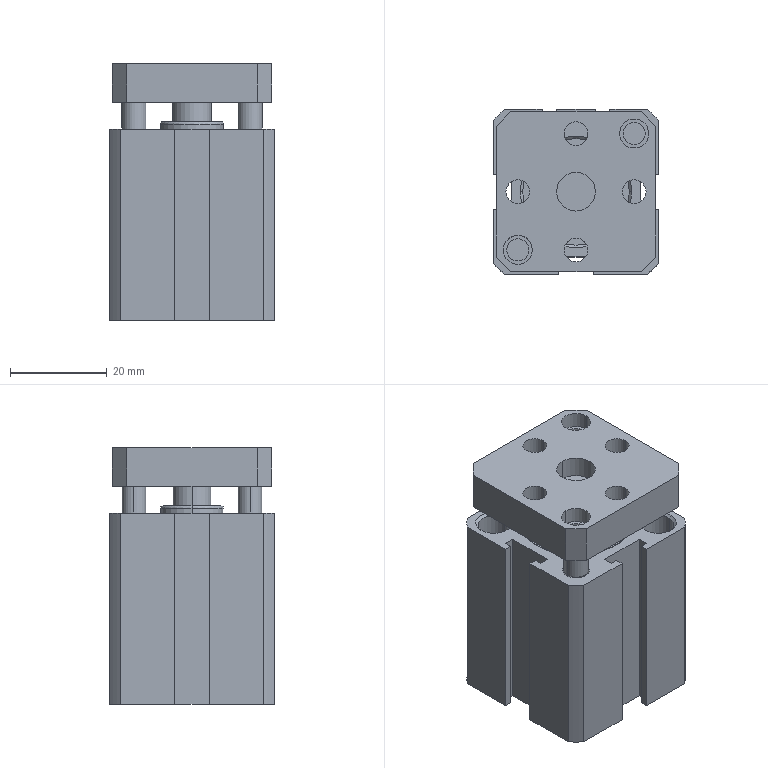Part | SolidWorks | features BaseBody 1 | 1 solid | 167 faces | box 34 x 34 x 53 mm | volume 43056 mm3 | cylinder 74 | plane 69 | cone 16 | spline 4 | torus 4 | commonest cylinder face diameters 4.917 x8 6.5 x8 22 x8 4.4 x6 1.5 x4 4.134 x4